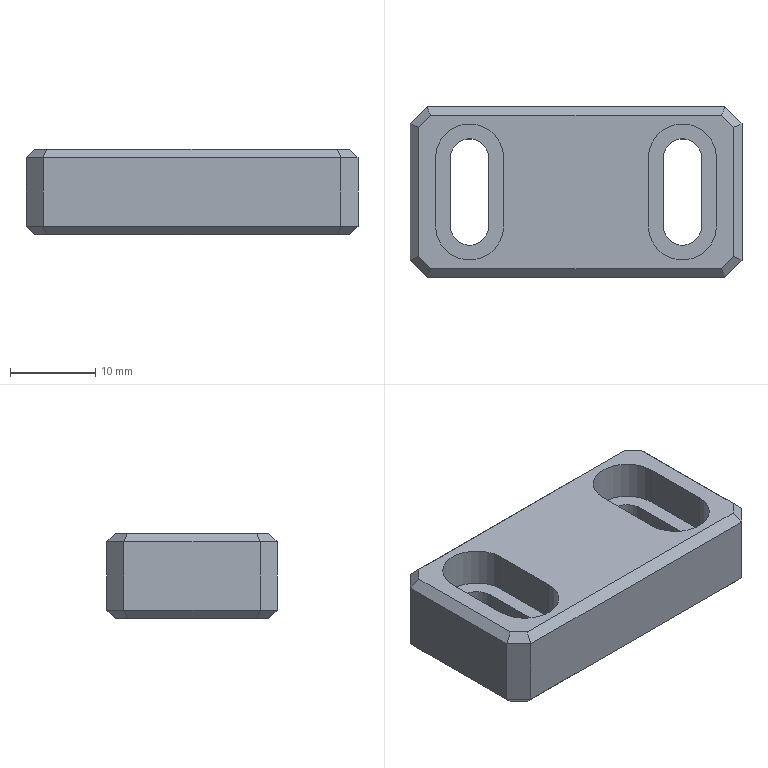Part | STEP file | TJ-DHQM-004-008 | 1 solid | 44 faces | box 39 x 20 x 10 mm | volume 5997 mm3 | plane 36 | cylinder 8 | commonest cylinder face diameters 4.5 x4 8 x4
STEP:
#1=CARTESIAN_POINT('',(-18.5,-7.586,0.));
#2=VERTEX_POINT('',#1);
#3=CARTESIAN_POINT('',(-18.5,7.586,0.));
#4=VERTEX_POINT('',#3);
#5=CARTESIAN_POINT('',(-18.5,8.,0.));
#6=DIRECTION('',(0.,1.,0.));
#7=VECTOR('',#6,1000.);
#8=LINE('',#5,#7);
#9=EDGE_CURVE('',#2,#4,#8,.T.);
#10=ORIENTED_EDGE('',*,*,#9,.T.);
#11=CARTESIAN_POINT('',(-17.086,9.,0.));
#12=VERTEX_POINT('',#11);
#13=CARTESIAN_POINT('',(-13.043,13.043,0.));
#14=DIRECTION('',(0.7071,0.7071,0.));
#15=VECTOR('',#14,1000.);
#16=LINE('',#13,#15);
#17=EDGE_CURVE('',#4,#12,#16,.T.);
#18=ORIENTED_EDGE('',*,*,#17,.T.);
#19=CARTESIAN_POINT('',(17.086,9.,0.));
#20=VERTEX_POINT('',#19);
#21=CARTESIAN_POINT('',(17.5,9.,0.));
#22=DIRECTION('',(1.,0.,0.));
#23=VECTOR('',#22,1000.);
#24=LINE('',#21,#23);
#25=EDGE_CURVE('',#12,#20,#24,.T.);
#26=ORIENTED_EDGE('',*,*,#25,.T.);
#27=CARTESIAN_POINT('',(18.5,7.586,0.));
#28=VERTEX_POINT('',#27);
#29=CARTESIAN_POINT('',(13.043,13.043,0.));
#30=DIRECTION('',(0.7071,-0.7071,0.));
#31=VECTOR('',#30,1000.);
#32=LINE('',#29,#31);
#33=EDGE_CURVE('',#20,#28,#32,.T.);
#34=ORIENTED_EDGE('',*,*,#33,.T.);
#35=CARTESIAN_POINT('',(18.5,-7.586,0.));
#36=VERTEX_POINT('',#35);
#37=CARTESIAN_POINT('',(18.5,-8.,0.));
#38=DIRECTION('',(0.,-1.,0.));
#39=VECTOR('',#38,1000.);
#40=LINE('',#37,#39);
#41=EDGE_CURVE('',#28,#36,#40,.T.);
#42=ORIENTED_EDGE('',*,*,#41,.T.);
#43=CARTESIAN_POINT('',(17.086,-9.,0.));
#44=VERTEX_POINT('',#43);
#45=CARTESIAN_POINT('',(13.043,-13.043,0.));
#46=DIRECTION('',(-0.7071,-0.7071,0.));
#47=VECTOR('',#46,1000.);
#48=LINE('',#45,#47);
#49=EDGE_CURVE('',#36,#44,#48,.T.);
#50=ORIENTED_EDGE('',*,*,#49,.T.);
#51=CARTESIAN_POINT('',(-17.086,-9.,0.));
#52=VERTEX_POINT('',#51);
#53=CARTESIAN_POINT('',(-17.5,-9.,0.));
#54=DIRECTION('',(-1.,0.,0.));
#55=VECTOR('',#54,1000.);
#56=LINE('',#53,#55);
#57=EDGE_CURVE('',#44,#52,#56,.T.);
#58=ORIENTED_EDGE('',*,*,#57,.T.);
#59=CARTESIAN_POINT('',(-13.043,-13.043,0.));
#60=DIRECTION('',(-0.7071,0.7071,0.));
#61=VECTOR('',#60,1000.);
#62=LINE('',#59,#61);
#63=EDGE_CURVE('',#52,#2,#62,.T.);
#64=ORIENTED_EDGE('',*,*,#63,.T.);
#65=EDGE_LOOP('',(#10,#18,#26,#34,#42,#50,#58,#64));
#66=FACE_OUTER_BOUND('',#65,.T.);
#67=CARTESIAN_POINT('',(-14.75,-4.,0.));
#68=VERTEX_POINT('',#67);
#69=CARTESIAN_POINT('',(-10.25,-4.,0.));
#70=VERTEX_POINT('',#69);
#71=CARTESIAN_POINT('',(-12.5,-4.,0.));
#72=DIRECTION('',(0.,0.,1.));
#73=DIRECTION('',(1.,0.,0.));
#74=AXIS2_PLACEMENT_3D('',#71,#72,#73);
#75=CIRCLE('',#74,2.25);
#76=EDGE_CURVE('',#68,#70,#75,.T.);
#77=ORIENTED_EDGE('',*,*,#76,.T.);
#78=CARTESIAN_POINT('',(-10.25,4.,0.));
#79=VERTEX_POINT('',#78);
#80=CARTESIAN_POINT('',(-10.25,-4.,0.));
#81=DIRECTION('',(0.,1.,0.));
#82=VECTOR('',#81,1000.);
#83=LINE('',#80,#82);
#84=EDGE_CURVE('',#70,#79,#83,.T.);
#85=ORIENTED_EDGE('',*,*,#84,.T.);
#86=CARTESIAN_POINT('',(-14.75,4.,0.));
#87=VERTEX_POINT('',#86);
#88=CARTESIAN_POINT('',(-12.5,4.,0.));
#89=DIRECTION('',(0.,0.,1.));
#90=DIRECTION('',(1.,0.,0.));
#91=AXIS2_PLACEMENT_3D('',#88,#89,#90);
#92=CIRCLE('',#91,2.25);
#93=EDGE_CURVE('',#79,#87,#92,.T.);
#94=ORIENTED_EDGE('',*,*,#93,.T.);
#95=CARTESIAN_POINT('',(-14.75,-4.,0.));
#96=DIRECTION('',(0.,1.,0.));
#97=VECTOR('',#96,1000.);
#98=LINE('',#95,#97);
#99=EDGE_CURVE('',#68,#87,#98,.T.);
#100=ORIENTED_EDGE('',*,*,#99,.F.);
#101=EDGE_LOOP('',(#77,#85,#94,#100));
#102=FACE_BOUND('',#101,.T.);
#103=CARTESIAN_POINT('',(14.75,-4.,0.));
#104=VERTEX_POINT('',#103);
#105=CARTESIAN_POINT('',(14.75,4.,0.));
#106=VERTEX_POINT('',#105);
#107=CARTESIAN_POINT('',(14.75,-4.,0.));
#108=DIRECTION('',(0.,1.,0.));
#109=VECTOR('',#108,1000.);
#110=LINE('',#107,#109);
#111=EDGE_CURVE('',#104,#106,#110,.T.);
#112=ORIENTED_EDGE('',*,*,#111,.T.);
#113=CARTESIAN_POINT('',(10.25,4.,0.));
#114=VERTEX_POINT('',#113);
#115=CARTESIAN_POINT('',(12.5,4.,0.));
#116=DIRECTION('',(0.,0.,1.));
#117=DIRECTION('',(1.,0.,0.));
#118=AXIS2_PLACEMENT_3D('',#115,#116,#117);
#119=CIRCLE('',#118,2.25);
#120=EDGE_CURVE('',#106,#114,#119,.T.);
#121=ORIENTED_EDGE('',*,*,#120,.T.);
#122=CARTESIAN_POINT('',(10.25,-4.,0.));
#123=VERTEX_POINT('',#122);
#124=CARTESIAN_POINT('',(10.25,-4.,0.));
#125=DIRECTION('',(0.,1.,0.));
#126=VECTOR('',#125,1000.);
#127=LINE('',#124,#126);
#128=EDGE_CURVE('',#123,#114,#127,.T.);
#129=ORIENTED_EDGE('',*,*,#128,.F.);
#130=CARTESIAN_POINT('',(12.5,-4.,0.));
#131=DIRECTION('',(0.,0.,1.));
#132=DIRECTION('',(1.,0.,0.));
#133=AXIS2_PLACEMENT_3D('',#130,#131,#132);
#134=CIRCLE('',#133,2.25);
#135=EDGE_CURVE('',#123,#104,#134,.T.);
#136=ORIENTED_EDGE('',*,*,#135,.T.);
#137=EDGE_LOOP('',(#112,#121,#129,#136));
#138=FACE_BOUND('',#137,.T.);
#139=CARTESIAN_POINT('',(0.,0.,0.));
#140=DIRECTION('',(0.,0.,-1.));
#141=DIRECTION('',(-1.,0.,0.));
#142=AXIS2_PLACEMENT_3D('',#139,#140,#141);
#143=PLANE('',#142);
#144=ADVANCED_FACE('',(#66,#102,#138),#143,.T.);
#145=CARTESIAN_POINT('',(19.5,-8.,9.));
#146=VERTEX_POINT('',#145);
#147=CARTESIAN_POINT('',(19.5,-8.,1.));
#148=VERTEX_POINT('',#147);
#149=CARTESIAN_POINT('',(19.5,-8.,10.));
#150=DIRECTION('',(0.,0.,-1.));
#151=VECTOR('',#150,1000.);
#152=LINE('',#149,#151);
#153=EDGE_CURVE('',#146,#148,#152,.T.);
#154=ORIENTED_EDGE('',*,*,#153,.T.);
#155=CARTESIAN_POINT('',(19.5,8.,1.));
#156=VERTEX_POINT('',#155);
#157=CARTESIAN_POINT('',(19.5,8.,1.));
#158=DIRECTION('',(0.,1.,0.));
#159=VECTOR('',#158,1000.);
#160=LINE('',#157,#159);
#161=EDGE_CURVE('',#148,#156,#160,.T.);
#162=ORIENTED_EDGE('',*,*,#161,.T.);
#163=CARTESIAN_POINT('',(19.5,8.,9.));
#164=VERTEX_POINT('',#163);
#165=CARTESIAN_POINT('',(19.5,8.,10.));
#166=DIRECTION('',(0.,0.,1.));
#167=VECTOR('',#166,1000.);
#168=LINE('',#165,#167);
#169=EDGE_CURVE('',#156,#164,#168,.T.);
#170=ORIENTED_EDGE('',*,*,#169,.T.);
#171=CARTESIAN_POINT('',(19.5,-10.,9.));
#172=DIRECTION('',(0.,-1.,0.));
#173=VECTOR('',#172,1000.);
#174=LINE('',#171,#173);
#175=EDGE_CURVE('',#164,#146,#174,.T.);
#176=ORIENTED_EDGE('',*,*,#175,.T.);
#177=EDGE_LOOP('',(#154,#162,#170,#176));
#178=FACE_OUTER_BOUND('',#177,.T.);
#179=CARTESIAN_POINT('',(19.5,-10.,10.));
#180=DIRECTION('',(-1.,0.,0.));
#181=DIRECTION('',(0.,0.,1.));
#182=AXIS2_PLACEMENT_3D('',#179,#180,#181);
#183=PLANE('',#182);
#184=ADVANCED_FACE('',(#178),#183,.F.);
#185=CARTESIAN_POINT('',(17.5,10.,9.));
#186=VERTEX_POINT('',#185);
#187=CARTESIAN_POINT('',(17.5,10.,1.));
#188=VERTEX_POINT('',#187);
#189=CARTESIAN_POINT('',(17.5,10.,10.));
#190=DIRECTION('',(0.,0.,-1.));
#191=VECTOR('',#190,1000.);
#192=LINE('',#189,#191);
#193=EDGE_CURVE('',#186,#188,#192,.T.);
#194=ORIENTED_EDGE('',*,*,#193,.T.);
#195=CARTESIAN_POINT('',(-17.5,10.,1.));
#196=VERTEX_POINT('',#195);
#197=CARTESIAN_POINT('',(-17.5,10.,1.));
#198=DIRECTION('',(-1.,0.,0.));
#199=VECTOR('',#198,1000.);
#200=LINE('',#197,#199);
#201=EDGE_CURVE('',#188,#196,#200,.T.);
#202=ORIENTED_EDGE('',*,*,#201,.T.);
#203=CARTESIAN_POINT('',(-17.5,10.,9.));
#204=VERTEX_POINT('',#203);
#205=CARTESIAN_POINT('',(-17.5,10.,10.));
#206=DIRECTION('',(0.,0.,1.));
#207=VECTOR('',#206,1000.);
#208=LINE('',#205,#207);
#209=EDGE_CURVE('',#196,#204,#208,.T.);
#210=ORIENTED_EDGE('',*,*,#209,.T.);
#211=CARTESIAN_POINT('',(-19.5,10.,9.));
#212=DIRECTION('',(1.,0.,0.));
#213=VECTOR('',#212,1000.);
#214=LINE('',#211,#213);
#215=EDGE_CURVE('',#204,#186,#214,.T.);
#216=ORIENTED_EDGE('',*,*,#215,.T.);
#217=EDGE_LOOP('',(#194,#202,#210,#216));
#218=FACE_OUTER_BOUND('',#217,.T.);
#219=CARTESIAN_POINT('',(-19.5,10.,10.));
#220=DIRECTION('',(0.,-1.,0.));
#221=DIRECTION('',(0.,0.,-1.));
#222=AXIS2_PLACEMENT_3D('',#219,#220,#221);
#223=PLANE('',#222);
#224=ADVANCED_FACE('',(#218),#223,.F.);
#225=CARTESIAN_POINT('',(-19.5,8.,9.));
#226=VERTEX_POINT('',#225);
#227=CARTESIAN_POINT('',(-19.5,8.,1.));
#228=VERTEX_POINT('',#227);
#229=CARTESIAN_POINT('',(-19.5,8.,10.));
#230=DIRECTION('',(0.,0.,-1.));
#231=VECTOR('',#230,1000.);
#232=LINE('',#229,#231);
#233=EDGE_CURVE('',#226,#228,#232,.T.);
#234=ORIENTED_EDGE('',*,*,#233,.T.);
#235=CARTESIAN_POINT('',(-19.5,-8.,1.));
#236=VERTEX_POINT('',#235);
#237=CARTESIAN_POINT('',(-19.5,-8.,1.));
#238=DIRECTION('',(0.,-1.,0.));
#239=VECTOR('',#238,1000.);
#240=LINE('',#237,#239);
#241=EDGE_CURVE('',#228,#236,#240,.T.);
#242=ORIENTED_EDGE('',*,*,#241,.T.);
#243=CARTESIAN_POINT('',(-19.5,-8.,9.));
#244=VERTEX_POINT('',#243);
#245=CARTESIAN_POINT('',(-19.5,-8.,10.));
#246=DIRECTION('',(0.,0.,1.));
#247=VECTOR('',#246,1000.);
#248=LINE('',#245,#247);
#249=EDGE_CURVE('',#236,#244,#248,.T.);
#250=ORIENTED_EDGE('',*,*,#249,.T.);
#251=CARTESIAN_POINT('',(-19.5,-10.,9.));
#252=DIRECTION('',(0.,1.,0.));
#253=VECTOR('',#252,1000.);
#254=LINE('',#251,#253);
#255=EDGE_CURVE('',#244,#226,#254,.T.);
#256=ORIENTED_EDGE('',*,*,#255,.T.);
#257=EDGE_LOOP('',(#234,#242,#250,#256));
#258=FACE_OUTER_BOUND('',#257,.T.);
#259=CARTESIAN_POINT('',(-19.5,-10.,10.));
#260=DIRECTION('',(1.,0.,0.));
#261=DIRECTION('',(0.,0.,-1.));
#262=AXIS2_PLACEMENT_3D('',#259,#260,#261);
#263=PLANE('',#262);
#264=ADVANCED_FACE('',(#258),#263,.F.);
#265=CARTESIAN_POINT('',(-17.5,-10.,9.));
#266=VERTEX_POINT('',#265);
#267=CARTESIAN_POINT('',(-17.5,-10.,1.));
#268=VERTEX_POINT('',#267);
#269=CARTESIAN_POINT('',(-17.5,-10.,10.));
#270=DIRECTION('',(0.,0.,-1.));
#271=VECTOR('',#270,1000.);
#272=LINE('',#269,#271);
#273=EDGE_CURVE('',#266,#268,#272,.T.);
#274=ORIENTED_EDGE('',*,*,#273,.T.);
#275=CARTESIAN_POINT('',(17.5,-10.,1.));
#276=VERTEX_POINT('',#275);
#277=CARTESIAN_POINT('',(17.5,-10.,1.));
#278=DIRECTION('',(1.,0.,0.));
#279=VECTOR('',#278,1000.);
#280=LINE('',#277,#279);
#281=EDGE_CURVE('',#268,#276,#280,.T.);
#282=ORIENTED_EDGE('',*,*,#281,.T.);
#283=CARTESIAN_POINT('',(17.5,-10.,9.));
#284=VERTEX_POINT('',#283);
#285=CARTESIAN_POINT('',(17.5,-10.,10.));
#286=DIRECTION('',(0.,0.,1.));
#287=VECTOR('',#286,1000.);
#288=LINE('',#285,#287);
#289=EDGE_CURVE('',#276,#284,#288,.T.);
#290=ORIENTED_EDGE('',*,*,#289,.T.);
#291=CARTESIAN_POINT('',(-19.5,-10.,9.));
#292=DIRECTION('',(-1.,0.,0.));
#293=VECTOR('',#292,1000.);
#294=LINE('',#291,#293);
#295=EDGE_CURVE('',#284,#266,#294,.T.);
#296=ORIENTED_EDGE('',*,*,#295,.T.);
#297=EDGE_LOOP('',(#274,#282,#290,#296));
#298=FACE_OUTER_BOUND('',#297,.T.);
#299=CARTESIAN_POINT('',(-19.5,-10.,10.));
#300=DIRECTION('',(0.,1.,0.));
#301=DIRECTION('',(0.,0.,1.));
#302=AXIS2_PLACEMENT_3D('',#299,#300,#301);
#303=PLANE('',#302);
#304=ADVANCED_FACE('',(#298),#303,.F.);
#305=CARTESIAN_POINT('',(-17.086,-9.,10.));
#306=VERTEX_POINT('',#305);
#307=CARTESIAN_POINT('',(17.086,-9.,10.));
#308=VERTEX_POINT('',#307);
#309=CARTESIAN_POINT('',(0.,-9.,10.));
#310=DIRECTION('',(1.,0.,0.));
#311=VECTOR('',#310,1000.);
#312=LINE('',#309,#311);
#313=EDGE_CURVE('',#306,#308,#312,.T.);
#314=ORIENTED_EDGE('',*,*,#313,.T.);
#315=CARTESIAN_POINT('',(18.5,-7.586,10.));
#316=VERTEX_POINT('',#315);
#317=CARTESIAN_POINT('',(18.793,-7.293,10.));
#318=DIRECTION('',(0.7071,0.7071,0.));
#319=VECTOR('',#318,1000.);
#320=LINE('',#317,#319);
#321=EDGE_CURVE('',#308,#316,#320,.T.);
#322=ORIENTED_EDGE('',*,*,#321,.T.);
#323=CARTESIAN_POINT('',(18.5,7.586,10.));
#324=VERTEX_POINT('',#323);
#325=CARTESIAN_POINT('',(18.5,0.,10.));
#326=DIRECTION('',(0.,1.,0.));
#327=VECTOR('',#326,1000.);
#328=LINE('',#325,#327);
#329=EDGE_CURVE('',#316,#324,#328,.T.);
#330=ORIENTED_EDGE('',*,*,#329,.T.);
#331=CARTESIAN_POINT('',(17.086,9.,10.));
#332=VERTEX_POINT('',#331);
#333=CARTESIAN_POINT('',(16.793,9.293,10.));
#334=DIRECTION('',(-0.7071,0.7071,0.));
#335=VECTOR('',#334,1000.);
#336=LINE('',#333,#335);
#337=EDGE_CURVE('',#324,#332,#336,.T.);
#338=ORIENTED_EDGE('',*,*,#337,.T.);
#339=CARTESIAN_POINT('',(-17.086,9.,10.));
#340=VERTEX_POINT('',#339);
#341=CARTESIAN_POINT('',(0.,9.,10.));
#342=DIRECTION('',(-1.,0.,0.));
#343=VECTOR('',#342,1000.);
#344=LINE('',#341,#343);
#345=EDGE_CURVE('',#332,#340,#344,.T.);
#346=ORIENTED_EDGE('',*,*,#345,.T.);
#347=CARTESIAN_POINT('',(-18.5,7.586,10.));
#348=VERTEX_POINT('',#347);
#349=CARTESIAN_POINT('',(-18.793,7.293,10.));
#350=DIRECTION('',(-0.7071,-0.7071,0.));
#351=VECTOR('',#350,1000.);
#352=LINE('',#349,#351);
#353=EDGE_CURVE('',#340,#348,#352,.T.);
#354=ORIENTED_EDGE('',*,*,#353,.T.);
#355=CARTESIAN_POINT('',(-18.5,-7.586,10.));
#356=VERTEX_POINT('',#355);
#357=CARTESIAN_POINT('',(-18.5,0.,10.));
#358=DIRECTION('',(0.,-1.,0.));
#359=VECTOR('',#358,1000.);
#360=LINE('',#357,#359);
#361=EDGE_CURVE('',#348,#356,#360,.T.);
#362=ORIENTED_EDGE('',*,*,#361,.T.);
#363=CARTESIAN_POINT('',(-16.793,-9.293,10.));
#364=DIRECTION('',(0.7071,-0.7071,0.));
#365=VECTOR('',#364,1000.);
#366=LINE('',#363,#365);
#367=EDGE_CURVE('',#356,#306,#366,.T.);
#368=ORIENTED_EDGE('',*,*,#367,.T.);
#369=EDGE_LOOP('',(#314,#322,#330,#338,#346,#354,#362,#368));
#370=FACE_OUTER_BOUND('',#369,.T.);
#371=CARTESIAN_POINT('',(-16.5,-4.,10.));
#372=VERTEX_POINT('',#371);
#373=CARTESIAN_POINT('',(-8.5,-4.,10.));
#374=VERTEX_POINT('',#373);
#375=CARTESIAN_POINT('',(-12.5,-4.,10.));
#376=DIRECTION('',(0.,0.,1.));
#377=DIRECTION('',(1.,0.,0.));
#378=AXIS2_PLACEMENT_3D('',#375,#376,#377);
#379=CIRCLE('',#378,4.);
#380=EDGE_CURVE('',#372,#374,#379,.T.);
#381=ORIENTED_EDGE('',*,*,#380,.F.);
#382=CARTESIAN_POINT('',(-16.5,4.,10.));
#383=VERTEX_POINT('',#382);
#384=CARTESIAN_POINT('',(-16.5,-4.,10.));
#385=DIRECTION('',(0.,1.,0.));
#386=VECTOR('',#385,1000.);
#387=LINE('',#384,#386);
#388=EDGE_CURVE('',#372,#383,#387,.T.);
#389=ORIENTED_EDGE('',*,*,#388,.T.);
#390=CARTESIAN_POINT('',(-8.5,4.,10.));
#391=VERTEX_POINT('',#390);
#392=CARTESIAN_POINT('',(-12.5,4.,10.));
#393=DIRECTION('',(0.,0.,1.));
#394=DIRECTION('',(1.,0.,0.));
#395=AXIS2_PLACEMENT_3D('',#392,#393,#394);
#396=CIRCLE('',#395,4.);
#397=EDGE_CURVE('',#391,#383,#396,.T.);
#398=ORIENTED_EDGE('',*,*,#397,.F.);
#399=CARTESIAN_POINT('',(-8.5,-4.,10.));
#400=DIRECTION('',(0.,1.,0.));
#401=VECTOR('',#400,1000.);
#402=LINE('',#399,#401);
#403=EDGE_CURVE('',#374,#391,#402,.T.);
#404=ORIENTED_EDGE('',*,*,#403,.F.);
#405=EDGE_LOOP('',(#381,#389,#398,#404));
#406=FACE_BOUND('',#405,.T.);
#407=CARTESIAN_POINT('',(16.5,4.,10.));
#408=VERTEX_POINT('',#407);
#409=CARTESIAN_POINT('',(8.5,4.,10.));
#410=VERTEX_POINT('',#409);
#411=CARTESIAN_POINT('',(12.5,4.,10.));
#412=DIRECTION('',(0.,0.,1.));
#413=DIRECTION('',(1.,0.,0.));
#414=AXIS2_PLACEMENT_3D('',#411,#412,#413);
#415=CIRCLE('',#414,4.);
#416=EDGE_CURVE('',#408,#410,#415,.T.);
#417=ORIENTED_EDGE('',*,*,#416,.F.);
#418=CARTESIAN_POINT('',(16.5,-4.,10.));
#419=VERTEX_POINT('',#418);
#420=CARTESIAN_POINT('',(16.5,-4.,10.));
#421=DIRECTION('',(0.,1.,0.));
#422=VECTOR('',#421,1000.);
#423=LINE('',#420,#422);
#424=EDGE_CURVE('',#419,#408,#423,.T.);
#425=ORIENTED_EDGE('',*,*,#424,.F.);
#426=CARTESIAN_POINT('',(8.5,-4.,10.));
#427=VERTEX_POINT('',#426);
#428=CARTESIAN_POINT('',(12.5,-4.,10.));
#429=DIRECTION('',(0.,0.,1.));
#430=DIRECTION('',(1.,0.,0.));
#431=AXIS2_PLACEMENT_3D('',#428,#429,#430);
#432=CIRCLE('',#431,4.);
#433=EDGE_CURVE('',#427,#419,#432,.T.);
#434=ORIENTED_EDGE('',*,*,#433,.F.);
#435=CARTESIAN_POINT('',(8.5,-4.,10.));
#436=DIRECTION('',(0.,1.,0.));
#437=VECTOR('',#436,1000.);
#438=LINE('',#435,#437);
#439=EDGE_CURVE('',#427,#410,#438,.T.);
#440=ORIENTED_EDGE('',*,*,#439,.T.);
#441=EDGE_LOOP('',(#417,#425,#434,#440));
#442=FACE_BOUND('',#441,.T.);
#443=CARTESIAN_POINT('',(0.,0.,10.));
#444=DIRECTION('',(0.,0.,-1.));
#445=DIRECTION('',(-1.,0.,0.));
#446=AXIS2_PLACEMENT_3D('',#443,#444,#445);
#447=PLANE('',#446);
#448=ADVANCED_FACE('',(#370,#406,#442),#447,.F.);
#449=ORIENTED_EDGE('',*,*,#169,.F.);
#450=CARTESIAN_POINT('',(17.5,10.,1.));
#451=DIRECTION('',(-0.7071,0.7071,0.));
#452=VECTOR('',#451,1000.);
#453=LINE('',#450,#452);
#454=EDGE_CURVE('',#156,#188,#453,.T.);
#455=ORIENTED_EDGE('',*,*,#454,.T.);
#456=ORIENTED_EDGE('',*,*,#193,.F.);
#457=CARTESIAN_POINT('',(19.5,8.,9.));
#458=DIRECTION('',(0.7071,-0.7071,0.));
#459=VECTOR('',#458,1000.);
#460=LINE('',#457,#459);
#461=EDGE_CURVE('',#186,#164,#460,.T.);
#462=ORIENTED_EDGE('',*,*,#461,.T.);
#463=EDGE_LOOP('',(#449,#455,#456,#462));
#464=FACE_OUTER_BOUND('',#463,.T.);
#465=CARTESIAN_POINT('',(17.5,10.,10.));
#466=DIRECTION('',(-0.7071,-0.7071,0.));
#467=DIRECTION('',(0.,0.,-1.));
#468=AXIS2_PLACEMENT_3D('',#465,#466,#467);
#469=PLANE('',#468);
#470=ADVANCED_FACE('',(#464),#469,.F.);
#471=ORIENTED_EDGE('',*,*,#289,.F.);
#472=CARTESIAN_POINT('',(19.5,-8.,1.));
#473=DIRECTION('',(0.7071,0.7071,0.));
#474=VECTOR('',#473,1000.);
#475=LINE('',#472,#474);
#476=EDGE_CURVE('',#276,#148,#475,.T.);
#477=ORIENTED_EDGE('',*,*,#476,.T.);
#478=ORIENTED_EDGE('',*,*,#153,.F.);
#479=CARTESIAN_POINT('',(17.5,-10.,9.));
#480=DIRECTION('',(-0.7071,-0.7071,0.));
#481=VECTOR('',#480,1000.);
#482=LINE('',#479,#481);
#483=EDGE_CURVE('',#146,#284,#482,.T.);
#484=ORIENTED_EDGE('',*,*,#483,.T.);
#485=EDGE_LOOP('',(#471,#477,#478,#484));
#486=FACE_OUTER_BOUND('',#485,.T.);
#487=CARTESIAN_POINT('',(19.5,-8.,10.));
#488=DIRECTION('',(-0.7071,0.7071,0.));
#489=DIRECTION('',(0.,0.,-1.));
#490=AXIS2_PLACEMENT_3D('',#487,#488,#489);
#491=PLANE('',#490);
#492=ADVANCED_FACE('',(#486),#491,.F.);
#493=ORIENTED_EDGE('',*,*,#249,.F.);
#494=CARTESIAN_POINT('',(-17.5,-10.,1.));
#495=DIRECTION('',(0.7071,-0.7071,0.));
#496=VECTOR('',#495,1000.);
#497=LINE('',#494,#496);
#498=EDGE_CURVE('',#236,#268,#497,.T.);
#499=ORIENTED_EDGE('',*,*,#498,.T.);
#500=ORIENTED_EDGE('',*,*,#273,.F.);
#501=CARTESIAN_POINT('',(-19.5,-8.,9.));
#502=DIRECTION('',(-0.7071,0.7071,0.));
#503=VECTOR('',#502,1000.);
#504=LINE('',#501,#503);
#505=EDGE_CURVE('',#266,#244,#504,.T.);
#506=ORIENTED_EDGE('',*,*,#505,.T.);
#507=EDGE_LOOP('',(#493,#499,#500,#506));
#508=FACE_OUTER_BOUND('',#507,.T.);
#509=CARTESIAN_POINT('',(-17.5,-10.,10.));
#510=DIRECTION('',(0.7071,0.7071,0.));
#511=DIRECTION('',(0.,0.,-1.));
#512=AXIS2_PLACEMENT_3D('',#509,#510,#511);
#513=PLANE('',#512);
#514=ADVANCED_FACE('',(#508),#513,.F.);
#515=ORIENTED_EDGE('',*,*,#209,.F.);
#516=CARTESIAN_POINT('',(-19.5,8.,1.));
#517=DIRECTION('',(-0.7071,-0.7071,0.));
#518=VECTOR('',#517,1000.);
#519=LINE('',#516,#518);
#520=EDGE_CURVE('',#196,#228,#519,.T.);
#521=ORIENTED_EDGE('',*,*,#520,.T.);
#522=ORIENTED_EDGE('',*,*,#233,.F.);
#523=CARTESIAN_POINT('',(-17.5,10.,9.));
#524=DIRECTION('',(0.7071,0.7071,0.));
#525=VECTOR('',#524,1000.);
#526=LINE('',#523,#525);
#527=EDGE_CURVE('',#226,#204,#526,.T.);
#528=ORIENTED_EDGE('',*,*,#527,.T.);
#529=EDGE_LOOP('',(#515,#521,#522,#528));
#530=FACE_OUTER_BOUND('',#529,.T.);
#531=CARTESIAN_POINT('',(-19.5,8.,10.));
#532=DIRECTION('',(0.7071,-0.7071,0.));
#533=DIRECTION('',(0.,0.,-1.));
#534=AXIS2_PLACEMENT_3D('',#531,#532,#533);
#535=PLANE('',#534);
#536=ADVANCED_FACE('',(#530),#535,.F.);
#537=ORIENTED_EDGE('',*,*,#120,.F.);
#538=CARTESIAN_POINT('',(14.75,4.,5.4));
#539=VERTEX_POINT('',#538);
#540=CARTESIAN_POINT('',(14.75,4.,0.));
#541=DIRECTION('',(0.,0.,-1.));
#542=VECTOR('',#541,1000.);
#543=LINE('',#540,#542);
#544=EDGE_CURVE('',#539,#106,#543,.T.);
#545=ORIENTED_EDGE('',*,*,#544,.F.);
#546=CARTESIAN_POINT('',(10.25,4.,5.4));
#547=VERTEX_POINT('',#546);
#548=CARTESIAN_POINT('',(12.5,4.,5.4));
#549=DIRECTION('',(0.,0.,1.));
#550=DIRECTION('',(1.,0.,0.));
#551=AXIS2_PLACEMENT_3D('',#548,#549,#550);
#552=CIRCLE('',#551,2.25);
#553=EDGE_CURVE('',#539,#547,#552,.T.);
#554=ORIENTED_EDGE('',*,*,#553,.T.);
#555=CARTESIAN_POINT('',(10.25,4.,10.));
#556=DIRECTION('',(0.,0.,1.));
#557=VECTOR('',#556,1000.);
#558=LINE('',#555,#557);
#559=EDGE_CURVE('',#114,#547,#558,.T.);
#560=ORIENTED_EDGE('',*,*,#559,.F.);
#561=EDGE_LOOP('',(#537,#545,#554,#560));
#562=FACE_OUTER_BOUND('',#561,.T.);
#563=CARTESIAN_POINT('',(12.5,4.,10.));
#564=DIRECTION('',(0.,0.,1.));
#565=DIRECTION('',(1.,0.,0.));
#566=AXIS2_PLACEMENT_3D('',#563,#564,#565);
#567=CYLINDRICAL_SURFACE('',#566,2.25);
#568=ADVANCED_FACE('',(#562),#567,.F.);
#569=CARTESIAN_POINT('',(8.5,-4.,5.4));
#570=VERTEX_POINT('',#569);
#571=CARTESIAN_POINT('',(8.5,4.,5.4));
#572=VERTEX_POINT('',#571);
#573=CARTESIAN_POINT('',(8.5,-4.,5.4));
#574=DIRECTION('',(0.,1.,0.));
#575=VECTOR('',#574,1000.);
#576=LINE('',#573,#575);
#577=EDGE_CURVE('',#570,#572,#576,.T.);
#578=ORIENTED_EDGE('',*,*,#577,.F.);
#579=CARTESIAN_POINT('',(16.5,-4.,5.4));
#580=VERTEX_POINT('',#579);
#581=CARTESIAN_POINT('',(12.5,-4.,5.4));
#582=DIRECTION('',(0.,0.,1.));
#583=DIRECTION('',(1.,0.,0.));
#584=AXIS2_PLACEMENT_3D('',#581,#582,#583);
#585=CIRCLE('',#584,4.);
#586=EDGE_CURVE('',#570,#580,#585,.T.);
#587=ORIENTED_EDGE('',*,*,#586,.T.);
#588=CARTESIAN_POINT('',(16.5,4.,5.4));
#589=VERTEX_POINT('',#588);
#590=CARTESIAN_POINT('',(16.5,-4.,5.4));
#591=DIRECTION('',(0.,1.,0.));
#592=VECTOR('',#591,1000.);
#593=LINE('',#590,#592);
#594=EDGE_CURVE('',#580,#589,#593,.T.);
#595=ORIENTED_EDGE('',*,*,#594,.T.);
#596=CARTESIAN_POINT('',(12.5,4.,5.4));
#597=DIRECTION('',(0.,0.,1.));
#598=DIRECTION('',(1.,0.,0.));
#599=AXIS2_PLACEMENT_3D('',#596,#597,#598);
#600=CIRCLE('',#599,4.);
#601=EDGE_CURVE('',#589,#572,#600,.T.);
#602=ORIENTED_EDGE('',*,*,#601,.T.);
#603=EDGE_LOOP('',(#578,#587,#595,#602));
#604=FACE_OUTER_BOUND('',#603,.T.);
#605=ORIENTED_EDGE('',*,*,#553,.F.);
#606=CARTESIAN_POINT('',(14.75,-4.,5.4));
#607=VERTEX_POINT('',#606);
#608=CARTESIAN_POINT('',(14.75,-4.,5.4));
#609=DIRECTION('',(0.,1.,0.));
#610=VECTOR('',#609,1000.);
#611=LINE('',#608,#610);
#612=EDGE_CURVE('',#607,#539,#611,.T.);
#613=ORIENTED_EDGE('',*,*,#612,.F.);
#614=CARTESIAN_POINT('',(10.25,-4.,5.4));
#615=VERTEX_POINT('',#614);
#616=CARTESIAN_POINT('',(12.5,-4.,5.4));
#617=DIRECTION('',(0.,0.,1.));
#618=DIRECTION('',(1.,0.,0.));
#619=AXIS2_PLACEMENT_3D('',#616,#617,#618);
#620=CIRCLE('',#619,2.25);
#621=EDGE_CURVE('',#615,#607,#620,.T.);
#622=ORIENTED_EDGE('',*,*,#621,.F.);
#623=CARTESIAN_POINT('',(10.25,-4.,5.4));
#624=DIRECTION('',(0.,1.,0.));
#625=VECTOR('',#624,1000.);
#626=LINE('',#623,#625);
#627=EDGE_CURVE('',#615,#547,#626,.T.);
#628=ORIENTED_EDGE('',*,*,#627,.T.);
#629=EDGE_LOOP('',(#605,#613,#622,#628));
#630=FACE_BOUND('',#629,.T.);
#631=CARTESIAN_POINT('',(14.75,4.,5.4));
#632=DIRECTION('',(0.,0.,-1.));
#633=DIRECTION('',(-1.,0.,0.));
#634=AXIS2_PLACEMENT_3D('',#631,#632,#633);
#635=PLANE('',#634);
#636=ADVANCED_FACE('',(#604,#630),#635,.F.);
#637=ORIENTED_EDGE('',*,*,#601,.F.);
#638=CARTESIAN_POINT('',(16.5,4.,5.4));
#639=DIRECTION('',(0.,0.,-1.));
#640=VECTOR('',#639,1000.);
#641=LINE('',#638,#640);
#642=EDGE_CURVE('',#408,#589,#641,.T.);
#643=ORIENTED_EDGE('',*,*,#642,.F.);
#644=ORIENTED_EDGE('',*,*,#416,.T.);
#645=CARTESIAN_POINT('',(8.5,4.,10.));
#646=DIRECTION('',(0.,0.,1.));
#647=VECTOR('',#646,1000.);
#648=LINE('',#645,#647);
#649=EDGE_CURVE('',#572,#410,#648,.T.);
#650=ORIENTED_EDGE('',*,*,#649,.F.);
#651=EDGE_LOOP('',(#637,#643,#644,#650));
#652=FACE_OUTER_BOUND('',#651,.T.);
#653=CARTESIAN_POINT('',(12.5,4.,10.));
#654=DIRECTION('',(0.,0.,1.));
#655=DIRECTION('',(1.,0.,0.));
#656=AXIS2_PLACEMENT_3D('',#653,#654,#655);
#657=CYLINDRICAL_SURFACE('',#656,4.);
#658=ADVANCED_FACE('',(#652),#657,.F.);
#659=ORIENTED_EDGE('',*,*,#621,.T.);
#660=CARTESIAN_POINT('',(14.75,-4.,0.));
#661=DIRECTION('',(0.,0.,-1.));
#662=VECTOR('',#661,1000.);
#663=LINE('',#660,#662);
#664=EDGE_CURVE('',#607,#104,#663,.T.);
#665=ORIENTED_EDGE('',*,*,#664,.T.);
#666=ORIENTED_EDGE('',*,*,#135,.F.);
#667=CARTESIAN_POINT('',(10.25,-4.,10.));
#668=DIRECTION('',(0.,0.,-1.));
#669=VECTOR('',#668,1000.);
#670=LINE('',#667,#669);
#671=EDGE_CURVE('',#615,#123,#670,.T.);
#672=ORIENTED_EDGE('',*,*,#671,.F.);
#673=EDGE_LOOP('',(#659,#665,#666,#672));
#674=FACE_OUTER_BOUND('',#673,.T.);
#675=CARTESIAN_POINT('',(12.5,-4.,10.));
#676=DIRECTION('',(0.,0.,1.));
#677=DIRECTION('',(1.,0.,0.));
#678=AXIS2_PLACEMENT_3D('',#675,#676,#677);
#679=CYLINDRICAL_SURFACE('',#678,2.25);
#680=ADVANCED_FACE('',(#674),#679,.F.);
#681=ORIENTED_EDGE('',*,*,#433,.T.);
#682=CARTESIAN_POINT('',(16.5,-4.,5.4));
#683=DIRECTION('',(0.,0.,-1.));
#684=VECTOR('',#683,1000.);
#685=LINE('',#682,#684);
#686=EDGE_CURVE('',#419,#580,#685,.T.);
#687=ORIENTED_EDGE('',*,*,#686,.T.);
#688=ORIENTED_EDGE('',*,*,#586,.F.);
#689=CARTESIAN_POINT('',(8.5,-4.,10.));
#690=DIRECTION('',(0.,0.,-1.));
#691=VECTOR('',#690,1000.);
#692=LINE('',#689,#691);
#693=EDGE_CURVE('',#427,#570,#692,.T.);
#694=ORIENTED_EDGE('',*,*,#693,.F.);
#695=EDGE_LOOP('',(#681,#687,#688,#694));
#696=FACE_OUTER_BOUND('',#695,.T.);
#697=CARTESIAN_POINT('',(12.5,-4.,10.));
#698=DIRECTION('',(0.,0.,1.));
#699=DIRECTION('',(1.,0.,0.));
#700=AXIS2_PLACEMENT_3D('',#697,#698,#699);
#701=CYLINDRICAL_SURFACE('',#700,4.);
#702=ADVANCED_FACE('',(#696),#701,.F.);
#703=ORIENTED_EDGE('',*,*,#649,.T.);
#704=ORIENTED_EDGE('',*,*,#439,.F.);
#705=ORIENTED_EDGE('',*,*,#693,.T.);
#706=ORIENTED_EDGE('',*,*,#577,.T.);
#707=EDGE_LOOP('',(#703,#704,#705,#706));
#708=FACE_OUTER_BOUND('',#707,.T.);
#709=CARTESIAN_POINT('',(8.5,-4.,10.));
#710=DIRECTION('',(-1.,0.,0.));
#711=DIRECTION('',(0.,-1.,0.));
#712=AXIS2_PLACEMENT_3D('',#709,#710,#711);
#713=PLANE('',#712);
#714=ADVANCED_FACE('',(#708),#713,.F.);
#715=ORIENTED_EDGE('',*,*,#559,.T.);
#716=ORIENTED_EDGE('',*,*,#627,.F.);
#717=ORIENTED_EDGE('',*,*,#671,.T.);
#718=ORIENTED_EDGE('',*,*,#128,.T.);
#719=EDGE_LOOP('',(#715,#716,#717,#718));
#720=FACE_OUTER_BOUND('',#719,.T.);
#721=CARTESIAN_POINT('',(10.25,-4.,10.));
#722=DIRECTION('',(-1.,0.,0.));
#723=DIRECTION('',(0.,-1.,0.));
#724=AXIS2_PLACEMENT_3D('',#721,#722,#723);
#725=PLANE('',#724);
#726=ADVANCED_FACE('',(#720),#725,.F.);
#727=ORIENTED_EDGE('',*,*,#544,.T.);
#728=ORIENTED_EDGE('',*,*,#111,.F.);
#729=ORIENTED_EDGE('',*,*,#664,.F.);
#730=ORIENTED_EDGE('',*,*,#612,.T.);
#731=EDGE_LOOP('',(#727,#728,#729,#730));
#732=FACE_OUTER_BOUND('',#731,.T.);
#733=CARTESIAN_POINT('',(14.75,-4.,0.));
#734=DIRECTION('',(1.,0.,0.));
#735=DIRECTION('',(0.,1.,0.));
#736=AXIS2_PLACEMENT_3D('',#733,#734,#735);
#737=PLANE('',#736);
#738=ADVANCED_FACE('',(#732),#737,.F.);
#739=ORIENTED_EDGE('',*,*,#642,.T.);
#740=ORIENTED_EDGE('',*,*,#594,.F.);
#741=ORIENTED_EDGE('',*,*,#686,.F.);
#742=ORIENTED_EDGE('',*,*,#424,.T.);
#743=EDGE_LOOP('',(#739,#740,#741,#742));
#744=FACE_OUTER_BOUND('',#743,.T.);
#745=CARTESIAN_POINT('',(16.5,-4.,5.4));
#746=DIRECTION('',(1.,0.,0.));
#747=DIRECTION('',(0.,1.,0.));
#748=AXIS2_PLACEMENT_3D('',#745,#746,#747);
#749=PLANE('',#748);
#750=ADVANCED_FACE('',(#744),#749,.F.);
#751=ORIENTED_EDGE('',*,*,#93,.F.);
#752=CARTESIAN_POINT('',(-10.25,4.,5.4));
#753=VERTEX_POINT('',#752);
#754=CARTESIAN_POINT('',(-10.25,4.,0.));
#755=DIRECTION('',(0.,0.,-1.));
#756=VECTOR('',#755,1000.);
#757=LINE('',#754,#756);
#758=EDGE_CURVE('',#753,#79,#757,.T.);
#759=ORIENTED_EDGE('',*,*,#758,.F.);
#760=CARTESIAN_POINT('',(-14.75,4.,5.4));
#761=VERTEX_POINT('',#760);
#762=CARTESIAN_POINT('',(-12.5,4.,5.4));
#763=DIRECTION('',(0.,0.,1.));
#764=DIRECTION('',(1.,0.,0.));
#765=AXIS2_PLACEMENT_3D('',#762,#763,#764);
#766=CIRCLE('',#765,2.25);
#767=EDGE_CURVE('',#753,#761,#766,.T.);
#768=ORIENTED_EDGE('',*,*,#767,.T.);
#769=CARTESIAN_POINT('',(-14.75,4.,10.));
#770=DIRECTION('',(0.,0.,1.));
#771=VECTOR('',#770,1000.);
#772=LINE('',#769,#771);
#773=EDGE_CURVE('',#87,#761,#772,.T.);
#774=ORIENTED_EDGE('',*,*,#773,.F.);
#775=EDGE_LOOP('',(#751,#759,#768,#774));
#776=FACE_OUTER_BOUND('',#775,.T.);
#777=CARTESIAN_POINT('',(-12.5,4.,10.));
#778=DIRECTION('',(0.,0.,1.));
#779=DIRECTION('',(1.,0.,0.));
#780=AXIS2_PLACEMENT_3D('',#777,#778,#779);
#781=CYLINDRICAL_SURFACE('',#780,2.25);
#782=ADVANCED_FACE('',(#776),#781,.F.);
#783=CARTESIAN_POINT('',(-16.5,-4.,5.4));
#784=VERTEX_POINT('',#783);
#785=CARTESIAN_POINT('',(-16.5,4.,5.4));
#786=VERTEX_POINT('',#785);
#787=CARTESIAN_POINT('',(-16.5,-4.,5.4));
#788=DIRECTION('',(0.,1.,0.));
#789=VECTOR('',#788,1000.);
#790=LINE('',#787,#789);
#791=EDGE_CURVE('',#784,#786,#790,.T.);
#792=ORIENTED_EDGE('',*,*,#791,.F.);
#793=CARTESIAN_POINT('',(-8.5,-4.,5.4));
#794=VERTEX_POINT('',#793);
#795=CARTESIAN_POINT('',(-12.5,-4.,5.4));
#796=DIRECTION('',(0.,0.,1.));
#797=DIRECTION('',(1.,0.,0.));
#798=AXIS2_PLACEMENT_3D('',#795,#796,#797);
#799=CIRCLE('',#798,4.);
#800=EDGE_CURVE('',#784,#794,#799,.T.);
#801=ORIENTED_EDGE('',*,*,#800,.T.);
#802=CARTESIAN_POINT('',(-8.5,4.,5.4));
#803=VERTEX_POINT('',#802);
#804=CARTESIAN_POINT('',(-8.5,-4.,5.4));
#805=DIRECTION('',(0.,1.,0.));
#806=VECTOR('',#805,1000.);
#807=LINE('',#804,#806);
#808=EDGE_CURVE('',#794,#803,#807,.T.);
#809=ORIENTED_EDGE('',*,*,#808,.T.);
#810=CARTESIAN_POINT('',(-12.5,4.,5.4));
#811=DIRECTION('',(0.,0.,1.));
#812=DIRECTION('',(1.,0.,0.));
#813=AXIS2_PLACEMENT_3D('',#810,#811,#812);
#814=CIRCLE('',#813,4.);
#815=EDGE_CURVE('',#803,#786,#814,.T.);
#816=ORIENTED_EDGE('',*,*,#815,.T.);
#817=EDGE_LOOP('',(#792,#801,#809,#816));
#818=FACE_OUTER_BOUND('',#817,.T.);
#819=ORIENTED_EDGE('',*,*,#767,.F.);
#820=CARTESIAN_POINT('',(-10.25,-4.,5.4));
#821=VERTEX_POINT('',#820);
#822=CARTESIAN_POINT('',(-10.25,-4.,5.4));
#823=DIRECTION('',(0.,1.,0.));
#824=VECTOR('',#823,1000.);
#825=LINE('',#822,#824);
#826=EDGE_CURVE('',#821,#753,#825,.T.);
#827=ORIENTED_EDGE('',*,*,#826,.F.);
#828=CARTESIAN_POINT('',(-14.75,-4.,5.4));
#829=VERTEX_POINT('',#828);
#830=CARTESIAN_POINT('',(-12.5,-4.,5.4));
#831=DIRECTION('',(0.,0.,1.));
#832=DIRECTION('',(1.,0.,0.));
#833=AXIS2_PLACEMENT_3D('',#830,#831,#832);
#834=CIRCLE('',#833,2.25);
#835=EDGE_CURVE('',#829,#821,#834,.T.);
#836=ORIENTED_EDGE('',*,*,#835,.F.);
#837=CARTESIAN_POINT('',(-14.75,-4.,5.4));
#838=DIRECTION('',(0.,1.,0.));
#839=VECTOR('',#838,1000.);
#840=LINE('',#837,#839);
#841=EDGE_CURVE('',#829,#761,#840,.T.);
#842=ORIENTED_EDGE('',*,*,#841,.T.);
#843=EDGE_LOOP('',(#819,#827,#836,#842));
#844=FACE_BOUND('',#843,.T.);
#845=CARTESIAN_POINT('',(-10.25,4.,5.4));
#846=DIRECTION('',(0.,0.,-1.));
#847=DIRECTION('',(-1.,0.,0.));
#848=AXIS2_PLACEMENT_3D('',#845,#846,#847);
#849=PLANE('',#848);
#850=ADVANCED_FACE('',(#818,#844),#849,.F.);
#851=ORIENTED_EDGE('',*,*,#815,.F.);
#852=CARTESIAN_POINT('',(-8.5,4.,5.4));
#853=DIRECTION('',(0.,0.,-1.));
#854=VECTOR('',#853,1000.);
#855=LINE('',#852,#854);
#856=EDGE_CURVE('',#391,#803,#855,.T.);
#857=ORIENTED_EDGE('',*,*,#856,.F.);
#858=ORIENTED_EDGE('',*,*,#397,.T.);
#859=CARTESIAN_POINT('',(-16.5,4.,10.));
#860=DIRECTION('',(0.,0.,1.));
#861=VECTOR('',#860,1000.);
#862=LINE('',#859,#861);
#863=EDGE_CURVE('',#786,#383,#862,.T.);
#864=ORIENTED_EDGE('',*,*,#863,.F.);
#865=EDGE_LOOP('',(#851,#857,#858,#864));
#866=FACE_OUTER_BOUND('',#865,.T.);
#867=CARTESIAN_POINT('',(-12.5,4.,10.));
#868=DIRECTION('',(0.,0.,1.));
#869=DIRECTION('',(1.,0.,0.));
#870=AXIS2_PLACEMENT_3D('',#867,#868,#869);
#871=CYLINDRICAL_SURFACE('',#870,4.);
#872=ADVANCED_FACE('',(#866),#871,.F.);
#873=ORIENTED_EDGE('',*,*,#835,.T.);
#874=CARTESIAN_POINT('',(-10.25,-4.,0.));
#875=DIRECTION('',(0.,0.,-1.));
#876=VECTOR('',#875,1000.);
#877=LINE('',#874,#876);
#878=EDGE_CURVE('',#821,#70,#877,.T.);
#879=ORIENTED_EDGE('',*,*,#878,.T.);
#880=ORIENTED_EDGE('',*,*,#76,.F.);
#881=CARTESIAN_POINT('',(-14.75,-4.,10.));
#882=DIRECTION('',(0.,0.,-1.));
#883=VECTOR('',#882,1000.);
#884=LINE('',#881,#883);
#885=EDGE_CURVE('',#829,#68,#884,.T.);
#886=ORIENTED_EDGE('',*,*,#885,.F.);
#887=EDGE_LOOP('',(#873,#879,#880,#886));
#888=FACE_OUTER_BOUND('',#887,.T.);
#889=CARTESIAN_POINT('',(-12.5,-4.,10.));
#890=DIRECTION('',(0.,0.,1.));
#891=DIRECTION('',(1.,0.,0.));
#892=AXIS2_PLACEMENT_3D('',#889,#890,#891);
#893=CYLINDRICAL_SURFACE('',#892,2.25);
#894=ADVANCED_FACE('',(#888),#893,.F.);
#895=ORIENTED_EDGE('',*,*,#380,.T.);
#896=CARTESIAN_POINT('',(-8.5,-4.,5.4));
#897=DIRECTION('',(0.,0.,-1.));
#898=VECTOR('',#897,1000.);
#899=LINE('',#896,#898);
#900=EDGE_CURVE('',#374,#794,#899,.T.);
#901=ORIENTED_EDGE('',*,*,#900,.T.);
#902=ORIENTED_EDGE('',*,*,#800,.F.);
#903=CARTESIAN_POINT('',(-16.5,-4.,10.));
#904=DIRECTION('',(0.,0.,-1.));
#905=VECTOR('',#904,1000.);
#906=LINE('',#903,#905);
#907=EDGE_CURVE('',#372,#784,#906,.T.);
#908=ORIENTED_EDGE('',*,*,#907,.F.);
#909=EDGE_LOOP('',(#895,#901,#902,#908));
#910=FACE_OUTER_BOUND('',#909,.T.);
#911=CARTESIAN_POINT('',(-12.5,-4.,10.));
#912=DIRECTION('',(0.,0.,1.));
#913=DIRECTION('',(1.,0.,0.));
#914=AXIS2_PLACEMENT_3D('',#911,#912,#913);
#915=CYLINDRICAL_SURFACE('',#914,4.);
#916=ADVANCED_FACE('',(#910),#915,.F.);
#917=ORIENTED_EDGE('',*,*,#863,.T.);
#918=ORIENTED_EDGE('',*,*,#388,.F.);
#919=ORIENTED_EDGE('',*,*,#907,.T.);
#920=ORIENTED_EDGE('',*,*,#791,.T.);
#921=EDGE_LOOP('',(#917,#918,#919,#920));
#922=FACE_OUTER_BOUND('',#921,.T.);
#923=CARTESIAN_POINT('',(-16.5,-4.,10.));
#924=DIRECTION('',(-1.,0.,0.));
#925=DIRECTION('',(0.,-1.,0.));
#926=AXIS2_PLACEMENT_3D('',#923,#924,#925);
#927=PLANE('',#926);
#928=ADVANCED_FACE('',(#922),#927,.F.);
#929=ORIENTED_EDGE('',*,*,#773,.T.);
#930=ORIENTED_EDGE('',*,*,#841,.F.);
#931=ORIENTED_EDGE('',*,*,#885,.T.);
#932=ORIENTED_EDGE('',*,*,#99,.T.);
#933=EDGE_LOOP('',(#929,#930,#931,#932));
#934=FACE_OUTER_BOUND('',#933,.T.);
#935=CARTESIAN_POINT('',(-14.75,-4.,10.));
#936=DIRECTION('',(-1.,0.,0.));
#937=DIRECTION('',(0.,-1.,0.));
#938=AXIS2_PLACEMENT_3D('',#935,#936,#937);
#939=PLANE('',#938);
#940=ADVANCED_FACE('',(#934),#939,.F.);
#941=ORIENTED_EDGE('',*,*,#758,.T.);
#942=ORIENTED_EDGE('',*,*,#84,.F.);
#943=ORIENTED_EDGE('',*,*,#878,.F.);
#944=ORIENTED_EDGE('',*,*,#826,.T.);
#945=EDGE_LOOP('',(#941,#942,#943,#944));
#946=FACE_OUTER_BOUND('',#945,.T.);
#947=CARTESIAN_POINT('',(-10.25,-4.,0.));
#948=DIRECTION('',(1.,0.,0.));
#949=DIRECTION('',(0.,1.,0.));
#950=AXIS2_PLACEMENT_3D('',#947,#948,#949);
#951=PLANE('',#950);
#952=ADVANCED_FACE('',(#946),#951,.F.);
#953=ORIENTED_EDGE('',*,*,#856,.T.);
#954=ORIENTED_EDGE('',*,*,#808,.F.);
#955=ORIENTED_EDGE('',*,*,#900,.F.);
#956=ORIENTED_EDGE('',*,*,#403,.T.);
#957=EDGE_LOOP('',(#953,#954,#955,#956));
#958=FACE_OUTER_BOUND('',#957,.T.);
#959=CARTESIAN_POINT('',(-8.5,-4.,5.4));
#960=DIRECTION('',(1.,0.,0.));
#961=DIRECTION('',(0.,1.,0.));
#962=AXIS2_PLACEMENT_3D('',#959,#960,#961);
#963=PLANE('',#962);
#964=ADVANCED_FACE('',(#958),#963,.F.);
#965=CARTESIAN_POINT('',(19.881,-8.158,1.381));
#966=DIRECTION('',(-0.6786,0.2811,-0.6786));
#967=VECTOR('',#966,1000.);
#968=LINE('',#965,#967);
#969=EDGE_CURVE('',#148,#36,#968,.T.);
#970=ORIENTED_EDGE('',*,*,#969,.F.);
#971=ORIENTED_EDGE('',*,*,#476,.F.);
#972=CARTESIAN_POINT('',(17.538,-10.091,1.091));
#973=DIRECTION('',(0.2811,-0.6786,0.6786));
#974=VECTOR('',#973,1000.);
#975=LINE('',#972,#974);
#976=EDGE_CURVE('',#44,#276,#975,.T.);
#977=ORIENTED_EDGE('',*,*,#976,.F.);
#978=ORIENTED_EDGE('',*,*,#49,.F.);
#979=EDGE_LOOP('',(#970,#971,#977,#978));
#980=FACE_OUTER_BOUND('',#979,.T.);
#981=CARTESIAN_POINT('',(13.043,-13.043,0.));
#982=DIRECTION('',(0.5,-0.5,-0.7071));
#983=DIRECTION('',(0.7071,0.7071,0.));
#984=AXIS2_PLACEMENT_3D('',#981,#982,#983);
#985=PLANE('',#984);
#986=ADVANCED_FACE('',(#980),#985,.T.);
#987=ORIENTED_EDGE('',*,*,#976,.T.);
#988=ORIENTED_EDGE('',*,*,#281,.F.);
#989=CARTESIAN_POINT('',(-17.658,-10.381,1.381));
#990=DIRECTION('',(-0.2811,-0.6786,0.6786));
#991=VECTOR('',#990,1000.);
#992=LINE('',#989,#991);
#993=EDGE_CURVE('',#52,#268,#992,.T.);
#994=ORIENTED_EDGE('',*,*,#993,.F.);
#995=ORIENTED_EDGE('',*,*,#57,.F.);
#996=EDGE_LOOP('',(#987,#988,#994,#995));
#997=FACE_OUTER_BOUND('',#996,.T.);
#998=CARTESIAN_POINT('',(-19.5,-10.,1.));
#999=DIRECTION('',(0.,-0.7071,-0.7071));
#1000=DIRECTION('',(-1.,0.,0.));
#1001=AXIS2_PLACEMENT_3D('',#998,#999,#1000);
#1002=PLANE('',#1001);
#1003=ADVANCED_FACE('',(#997),#1002,.T.);
#1004=ORIENTED_EDGE('',*,*,#969,.T.);
#1005=ORIENTED_EDGE('',*,*,#41,.F.);
#1006=CARTESIAN_POINT('',(17.028,6.976,-1.472));
#1007=DIRECTION('',(-0.6786,-0.2811,-0.6786));
#1008=VECTOR('',#1007,1000.);
#1009=LINE('',#1006,#1008);
#1010=EDGE_CURVE('',#156,#28,#1009,.T.);
#1011=ORIENTED_EDGE('',*,*,#1010,.F.);
#1012=ORIENTED_EDGE('',*,*,#161,.F.);
#1013=EDGE_LOOP('',(#1004,#1005,#1011,#1012));
#1014=FACE_OUTER_BOUND('',#1013,.T.);
#1015=CARTESIAN_POINT('',(19.5,-10.,1.));
#1016=DIRECTION('',(0.7071,0.,-0.7071));
#1017=DIRECTION('',(0.,-1.,0.));
#1018=AXIS2_PLACEMENT_3D('',#1015,#1016,#1017);
#1019=PLANE('',#1018);
#1020=ADVANCED_FACE('',(#1014),#1019,.T.);
#1021=ORIENTED_EDGE('',*,*,#993,.T.);
#1022=ORIENTED_EDGE('',*,*,#498,.F.);
#1023=CARTESIAN_POINT('',(-17.028,-6.976,-1.472));
#1024=DIRECTION('',(-0.6786,-0.2811,0.6786));
#1025=VECTOR('',#1024,1000.);
#1026=LINE('',#1023,#1025);
#1027=EDGE_CURVE('',#2,#236,#1026,.T.);
#1028=ORIENTED_EDGE('',*,*,#1027,.F.);
#1029=ORIENTED_EDGE('',*,*,#63,.F.);
#1030=EDGE_LOOP('',(#1021,#1022,#1028,#1029));
#1031=FACE_OUTER_BOUND('',#1030,.T.);
#1032=CARTESIAN_POINT('',(-13.043,-13.043,0.));
#1033=DIRECTION('',(-0.5,-0.5,-0.7071));
#1034=DIRECTION('',(0.7071,-0.7071,0.));
#1035=AXIS2_PLACEMENT_3D('',#1032,#1033,#1034);
#1036=PLANE('',#1035);
#1037=ADVANCED_FACE('',(#1031),#1036,.T.);
#1038=ORIENTED_EDGE('',*,*,#1010,.T.);
#1039=ORIENTED_EDGE('',*,*,#33,.F.);
#1040=CARTESIAN_POINT('',(14.577,2.942,-6.058));
#1041=DIRECTION('',(-0.2811,-0.6786,-0.6786));
#1042=VECTOR('',#1041,1000.);
#1043=LINE('',#1040,#1042);
#1044=EDGE_CURVE('',#188,#20,#1043,.T.);
#1045=ORIENTED_EDGE('',*,*,#1044,.F.);
#1046=ORIENTED_EDGE('',*,*,#454,.F.);
#1047=EDGE_LOOP('',(#1038,#1039,#1045,#1046));
#1048=FACE_OUTER_BOUND('',#1047,.T.);
#1049=CARTESIAN_POINT('',(13.043,13.043,0.));
#1050=DIRECTION('',(0.5,0.5,-0.7071));
#1051=DIRECTION('',(-0.7071,0.7071,0.));
#1052=AXIS2_PLACEMENT_3D('',#1049,#1050,#1051);
#1053=PLANE('',#1052);
#1054=ADVANCED_FACE('',(#1048),#1053,.T.);
#1055=ORIENTED_EDGE('',*,*,#1027,.T.);
#1056=ORIENTED_EDGE('',*,*,#241,.F.);
#1057=CARTESIAN_POINT('',(-16.067,6.578,-2.433));
#1058=DIRECTION('',(-0.6786,0.2811,0.6786));
#1059=VECTOR('',#1058,1000.);
#1060=LINE('',#1057,#1059);
#1061=EDGE_CURVE('',#4,#228,#1060,.T.);
#1062=ORIENTED_EDGE('',*,*,#1061,.F.);
#1063=ORIENTED_EDGE('',*,*,#9,.F.);
#1064=EDGE_LOOP('',(#1055,#1056,#1062,#1063));
#1065=FACE_OUTER_BOUND('',#1064,.T.);
#1066=CARTESIAN_POINT('',(-19.5,-10.,1.));
#1067=DIRECTION('',(-0.7071,0.,-0.7071));
#1068=DIRECTION('',(0.,1.,0.));
#1069=AXIS2_PLACEMENT_3D('',#1066,#1067,#1068);
#1070=PLANE('',#1069);
#1071=ADVANCED_FACE('',(#1065),#1070,.T.);
#1072=ORIENTED_EDGE('',*,*,#1044,.T.);
#1073=ORIENTED_EDGE('',*,*,#25,.F.);
#1074=CARTESIAN_POINT('',(-17.658,10.381,1.381));
#1075=DIRECTION('',(0.2811,-0.6786,-0.6786));
#1076=VECTOR('',#1075,1000.);
#1077=LINE('',#1074,#1076);
#1078=EDGE_CURVE('',#196,#12,#1077,.T.);
#1079=ORIENTED_EDGE('',*,*,#1078,.F.);
#1080=ORIENTED_EDGE('',*,*,#201,.F.);
#1081=EDGE_LOOP('',(#1072,#1073,#1079,#1080));
#1082=FACE_OUTER_BOUND('',#1081,.T.);
#1083=CARTESIAN_POINT('',(-19.5,10.,1.));
#1084=DIRECTION('',(0.,0.7071,-0.7071));
#1085=DIRECTION('',(1.,0.,0.));
#1086=AXIS2_PLACEMENT_3D('',#1083,#1084,#1085);
#1087=PLANE('',#1086);
#1088=ADVANCED_FACE('',(#1082),#1087,.T.);
#1089=ORIENTED_EDGE('',*,*,#1061,.T.);
#1090=ORIENTED_EDGE('',*,*,#520,.F.);
#1091=ORIENTED_EDGE('',*,*,#1078,.T.);
#1092=ORIENTED_EDGE('',*,*,#17,.F.);
#1093=EDGE_LOOP('',(#1089,#1090,#1091,#1092));
#1094=FACE_OUTER_BOUND('',#1093,.T.);
#1095=CARTESIAN_POINT('',(-13.043,13.043,0.));
#1096=DIRECTION('',(-0.5,0.5,-0.7071));
#1097=DIRECTION('',(-0.7071,-0.7071,0.));
#1098=AXIS2_PLACEMENT_3D('',#1095,#1096,#1097);
#1099=PLANE('',#1098);
#1100=ADVANCED_FACE('',(#1094),#1099,.T.);
#1101=CARTESIAN_POINT('',(-17.538,10.091,8.909));
#1102=DIRECTION('',(0.2811,-0.6786,0.6786));
#1103=VECTOR('',#1102,1000.);
#1104=LINE('',#1101,#1103);
#1105=EDGE_CURVE('',#204,#340,#1104,.T.);
#1106=ORIENTED_EDGE('',*,*,#1105,.F.);
#1107=ORIENTED_EDGE('',*,*,#527,.F.);
#1108=CARTESIAN_POINT('',(-17.053,6.986,11.447));
#1109=DIRECTION('',(-0.6786,0.2811,-0.6786));
#1110=VECTOR('',#1109,1000.);
#1111=LINE('',#1108,#1110);
#1112=EDGE_CURVE('',#348,#226,#1111,.T.);
#1113=ORIENTED_EDGE('',*,*,#1112,.F.);
#1114=ORIENTED_EDGE('',*,*,#353,.F.);
#1115=EDGE_LOOP('',(#1106,#1107,#1113,#1114));
#1116=FACE_OUTER_BOUND('',#1115,.T.);
#1117=CARTESIAN_POINT('',(-13.043,13.043,10.));
#1118=DIRECTION('',(0.5,-0.5,-0.7071));
#1119=DIRECTION('',(-0.7071,-0.7071,0.));
#1120=AXIS2_PLACEMENT_3D('',#1117,#1118,#1119);
#1121=PLANE('',#1120);
#1122=ADVANCED_FACE('',(#1116),#1121,.F.);
#1123=ORIENTED_EDGE('',*,*,#1112,.T.);
#1124=ORIENTED_EDGE('',*,*,#255,.F.);
#1125=CARTESIAN_POINT('',(-17.028,-6.976,11.472));
#1126=DIRECTION('',(-0.6786,-0.2811,-0.6786));
#1127=VECTOR('',#1126,1000.);
#1128=LINE('',#1125,#1127);
#1129=EDGE_CURVE('',#356,#244,#1128,.T.);
#1130=ORIENTED_EDGE('',*,*,#1129,.F.);
#1131=ORIENTED_EDGE('',*,*,#361,.F.);
#1132=EDGE_LOOP('',(#1123,#1124,#1130,#1131));
#1133=FACE_OUTER_BOUND('',#1132,.T.);
#1134=CARTESIAN_POINT('',(-18.5,0.,10.));
#1135=DIRECTION('',(0.7071,0.,-0.7071));
#1136=DIRECTION('',(0.,-1.,0.));
#1137=AXIS2_PLACEMENT_3D('',#1134,#1135,#1136);
#1138=PLANE('',#1137);
#1139=ADVANCED_FACE('',(#1133),#1138,.F.);
#1140=ORIENTED_EDGE('',*,*,#1105,.T.);
#1141=ORIENTED_EDGE('',*,*,#345,.F.);
#1142=CARTESIAN_POINT('',(15.736,5.741,13.259));
#1143=DIRECTION('',(-0.2811,-0.6786,0.6786));
#1144=VECTOR('',#1143,1000.);
#1145=LINE('',#1142,#1144);
#1146=EDGE_CURVE('',#186,#332,#1145,.T.);
#1147=ORIENTED_EDGE('',*,*,#1146,.F.);
#1148=ORIENTED_EDGE('',*,*,#215,.F.);
#1149=EDGE_LOOP('',(#1140,#1141,#1147,#1148));
#1150=FACE_OUTER_BOUND('',#1149,.T.);
#1151=CARTESIAN_POINT('',(0.,9.,10.));
#1152=DIRECTION('',(0.,-0.7071,-0.7071));
#1153=DIRECTION('',(-1.,0.,0.));
#1154=AXIS2_PLACEMENT_3D('',#1151,#1152,#1153);
#1155=PLANE('',#1154);
#1156=ADVANCED_FACE('',(#1150),#1155,.F.);
#1157=ORIENTED_EDGE('',*,*,#1129,.T.);
#1158=ORIENTED_EDGE('',*,*,#505,.F.);
#1159=CARTESIAN_POINT('',(-15.736,-5.741,13.259));
#1160=DIRECTION('',(-0.2811,-0.6786,-0.6786));
#1161=VECTOR('',#1160,1000.);
#1162=LINE('',#1159,#1161);
#1163=EDGE_CURVE('',#306,#266,#1162,.T.);
#1164=ORIENTED_EDGE('',*,*,#1163,.F.);
#1165=ORIENTED_EDGE('',*,*,#367,.F.);
#1166=EDGE_LOOP('',(#1157,#1158,#1164,#1165));
#1167=FACE_OUTER_BOUND('',#1166,.T.);
#1168=CARTESIAN_POINT('',(-13.043,-13.043,10.));
#1169=DIRECTION('',(0.5,0.5,-0.7071));
#1170=DIRECTION('',(0.7071,-0.7071,0.));
#1171=AXIS2_PLACEMENT_3D('',#1168,#1169,#1170);
#1172=PLANE('',#1171);
#1173=ADVANCED_FACE('',(#1167),#1172,.F.);
#1174=ORIENTED_EDGE('',*,*,#1146,.T.);
#1175=ORIENTED_EDGE('',*,*,#337,.F.);
#1176=CARTESIAN_POINT('',(17.028,6.976,11.472));
#1177=DIRECTION('',(-0.6786,-0.2811,0.6786));
#1178=VECTOR('',#1177,1000.);
#1179=LINE('',#1176,#1178);
#1180=EDGE_CURVE('',#164,#324,#1179,.T.);
#1181=ORIENTED_EDGE('',*,*,#1180,.F.);
#1182=ORIENTED_EDGE('',*,*,#461,.F.);
#1183=EDGE_LOOP('',(#1174,#1175,#1181,#1182));
#1184=FACE_OUTER_BOUND('',#1183,.T.);
#1185=CARTESIAN_POINT('',(13.043,13.043,10.));
#1186=DIRECTION('',(-0.5,-0.5,-0.7071));
#1187=DIRECTION('',(-0.7071,0.7071,0.));
#1188=AXIS2_PLACEMENT_3D('',#1185,#1186,#1187);
#1189=PLANE('',#1188);
#1190=ADVANCED_FACE('',(#1184),#1189,.F.);
#1191=ORIENTED_EDGE('',*,*,#1163,.T.);
#1192=ORIENTED_EDGE('',*,*,#295,.F.);
#1193=CARTESIAN_POINT('',(15.736,-5.741,13.259));
#1194=DIRECTION('',(0.2811,-0.6786,-0.6786));
#1195=VECTOR('',#1194,1000.);
#1196=LINE('',#1193,#1195);
#1197=EDGE_CURVE('',#308,#284,#1196,.T.);
#1198=ORIENTED_EDGE('',*,*,#1197,.F.);
#1199=ORIENTED_EDGE('',*,*,#313,.F.);
#1200=EDGE_LOOP('',(#1191,#1192,#1198,#1199));
#1201=FACE_OUTER_BOUND('',#1200,.T.);
#1202=CARTESIAN_POINT('',(0.,-9.,10.));
#1203=DIRECTION('',(0.,0.7071,-0.7071));
#1204=DIRECTION('',(1.,0.,0.));
#1205=AXIS2_PLACEMENT_3D('',#1202,#1203,#1204);
#1206=PLANE('',#1205);
#1207=ADVANCED_FACE('',(#1201),#1206,.F.);
#1208=ORIENTED_EDGE('',*,*,#1180,.T.);
#1209=ORIENTED_EDGE('',*,*,#329,.F.);
#1210=CARTESIAN_POINT('',(17.053,-6.986,11.447));
#1211=DIRECTION('',(-0.6786,0.2811,0.6786));
#1212=VECTOR('',#1211,1000.);
#1213=LINE('',#1210,#1212);
#1214=EDGE_CURVE('',#146,#316,#1213,.T.);
#1215=ORIENTED_EDGE('',*,*,#1214,.F.);
#1216=ORIENTED_EDGE('',*,*,#175,.F.);
#1217=EDGE_LOOP('',(#1208,#1209,#1215,#1216));
#1218=FACE_OUTER_BOUND('',#1217,.T.);
#1219=CARTESIAN_POINT('',(18.5,0.,10.));
#1220=DIRECTION('',(-0.7071,0.,-0.7071));
#1221=DIRECTION('',(0.,1.,0.));
#1222=AXIS2_PLACEMENT_3D('',#1219,#1220,#1221);
#1223=PLANE('',#1222);
#1224=ADVANCED_FACE('',(#1218),#1223,.F.);
#1225=ORIENTED_EDGE('',*,*,#1197,.T.);
#1226=ORIENTED_EDGE('',*,*,#483,.F.);
#1227=ORIENTED_EDGE('',*,*,#1214,.T.);
#1228=ORIENTED_EDGE('',*,*,#321,.F.);
#1229=EDGE_LOOP('',(#1225,#1226,#1227,#1228));
#1230=FACE_OUTER_BOUND('',#1229,.T.);
#1231=CARTESIAN_POINT('',(13.043,-13.043,10.));
#1232=DIRECTION('',(-0.5,0.5,-0.7071));
#1233=DIRECTION('',(0.7071,0.7071,0.));
#1234=AXIS2_PLACEMENT_3D('',#1231,#1232,#1233);
#1235=PLANE('',#1234);
#1236=ADVANCED_FACE('',(#1230),#1235,.F.);
#1237=CLOSED_SHELL('',(#144,#184,#224,#264,#304,#448,#470,#492,#514,#536,#568,#636,#658,#680,#702,#714,#726,#738,#750,#782,#850,#872,#894,#916,#928,#940,#952,#964,#986,#1003,#1020,#1037,#1054,#1071,#1088,#1100,#1122,#1139,#1156,#1173,#1190,#1207,#1224,#1236));
#1238=MANIFOLD_SOLID_BREP('',#1237);
#1239=CARTESIAN_POINT('',(0.,0.,0.));
#1240=DIRECTION('',(0.,0.,1.));
#1241=DIRECTION('',(1.,0.,0.));
#1242=AXIS2_PLACEMENT_3D('',#1239,#1240,#1241);
#1243=(LENGTH_UNIT()NAMED_UNIT(*)SI_UNIT(.MILLI.,.METRE.));
#1244=UNCERTAINTY_MEASURE_WITH_UNIT(LENGTH_MEASURE(0.00001),#1243,'','');
#1245=(NAMED_UNIT(*)PLANE_ANGLE_UNIT()SI_UNIT($,.RADIAN.));
#1246=(NAMED_UNIT(*)SI_UNIT($,.STERADIAN.)SOLID_ANGLE_UNIT());
#1247=(GEOMETRIC_REPRESENTATION_CONTEXT(3)GLOBAL_UNCERTAINTY_ASSIGNED_CONTEXT((#1244))GLOBAL_UNIT_ASSIGNED_CONTEXT((#1243,#1245,#1246))REPRESENTATION_CONTEXT('',''));
#1248=ADVANCED_BREP_SHAPE_REPRESENTATION('',(#1238,#1242),#1247);